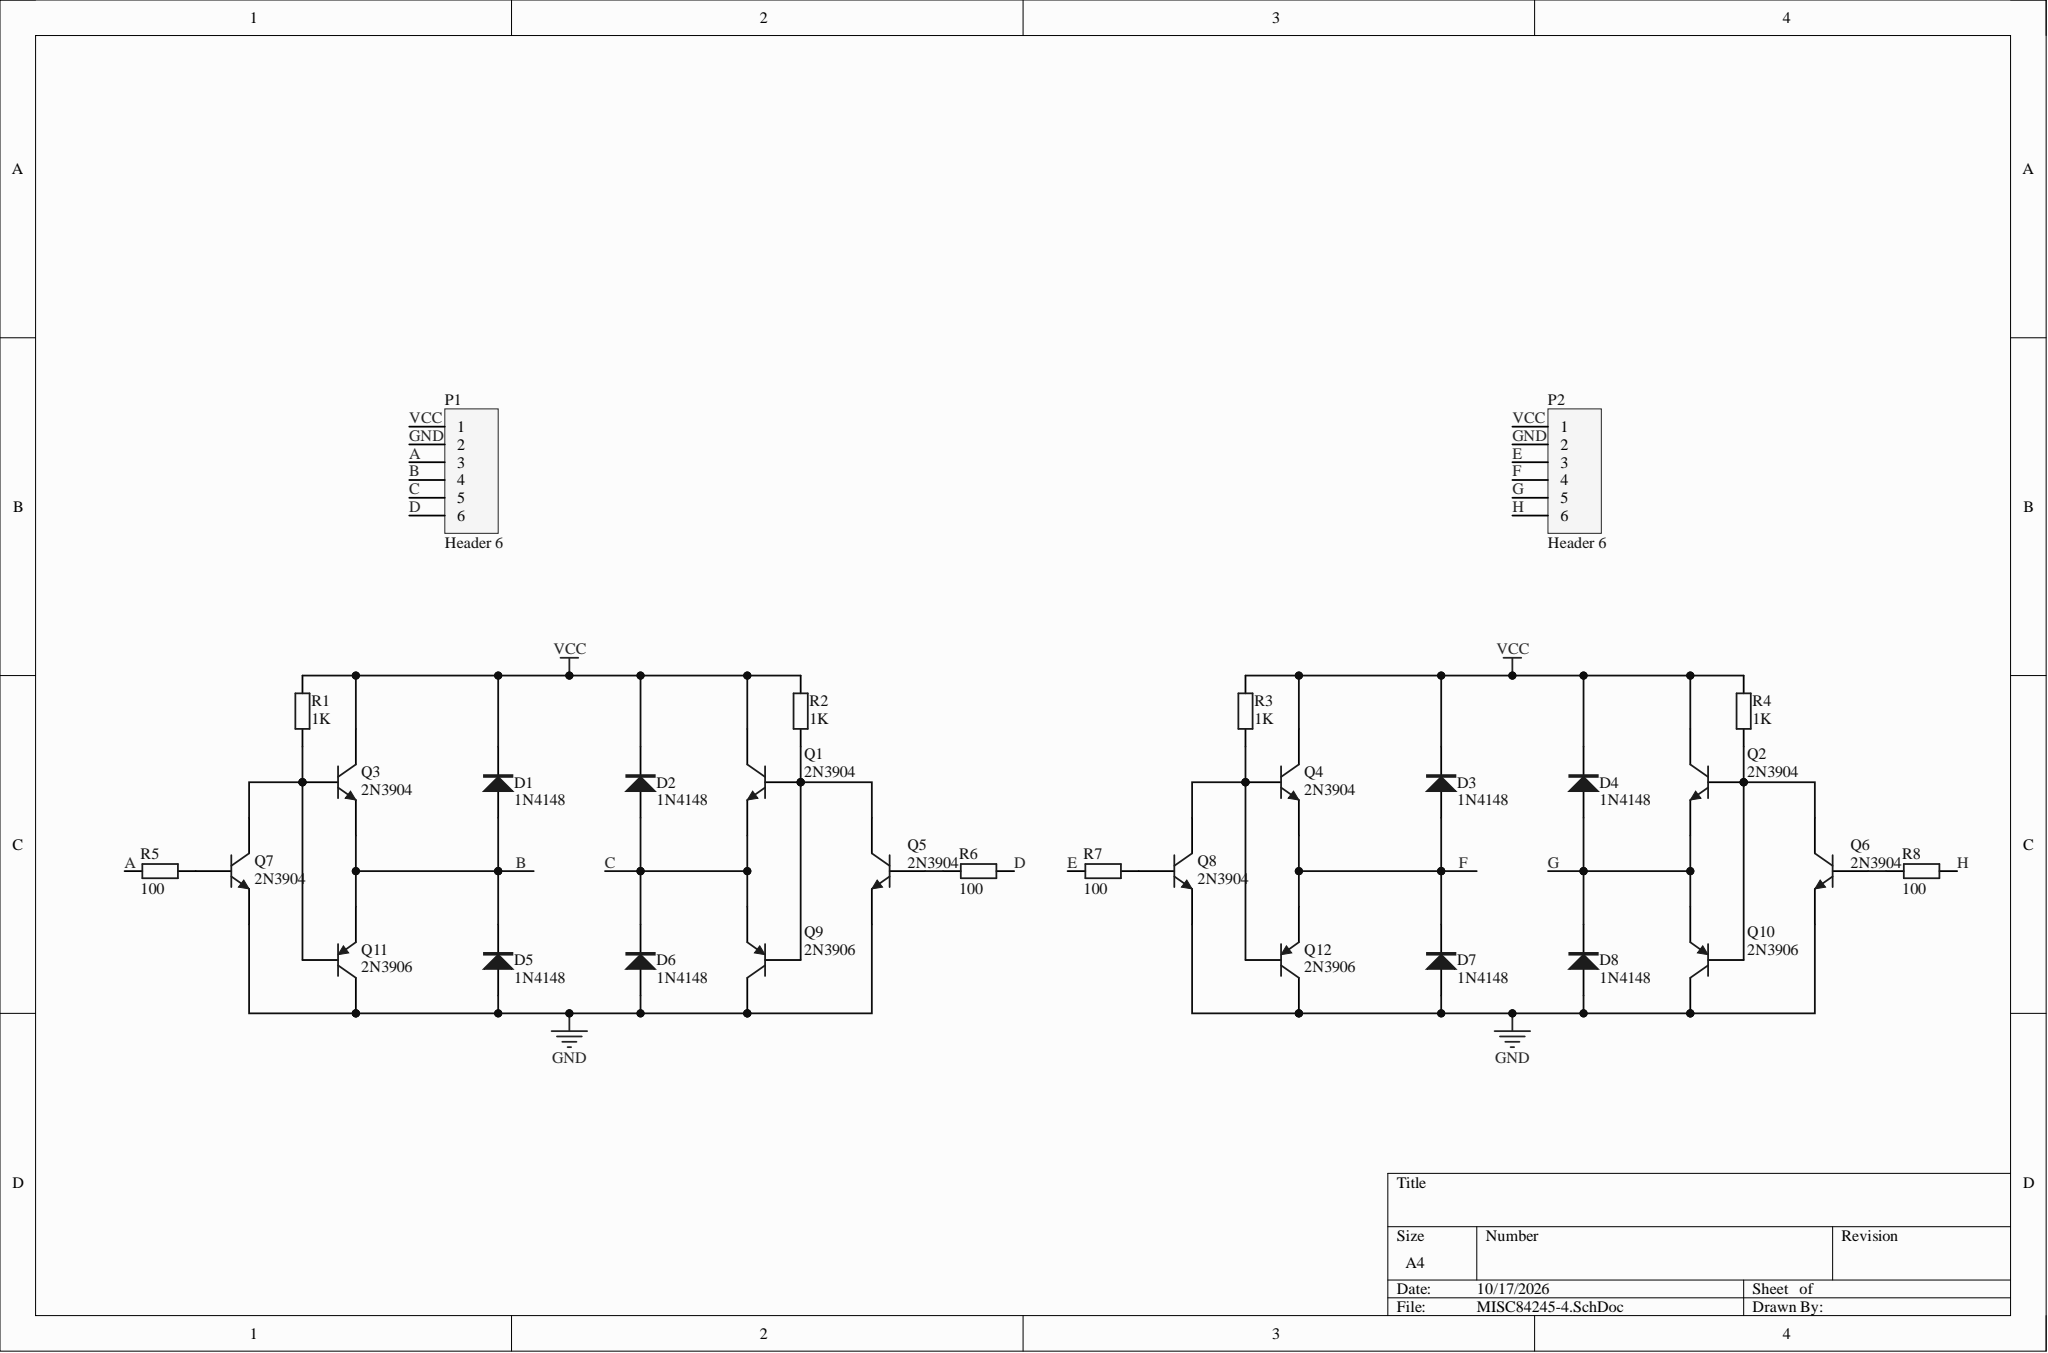Circuit board | Altium Designer | 30 parts | 18 nets
Bill of materials:
Comment,Description,Designator,Footprint,LibRef,Quantity
"1N4148","Switching diode","D1, D2, D3, D4, D5, D6, D7, D8","DO-41","1N4148","8"
"Header 6","Header, 6-Pin","P1, P2","HDR1X6","Header 6","2"
"2N3904","NPN General Purpose Amplifier","Q1, Q2, Q3, Q4, Q5, Q6, Q7, Q8","TO-92A","2N3904","8"
"2N3906","PNP General Purpose Amplifier","Q9, Q10, Q11, Q12","TO-92A","2N3906","4"
"1K","Color-band resistor","R1, R2, R3, R4","RS 1/4W","R-S","4"
"100","Color-band resistor","R5, R6, R7, R8","RS 1/4W","R-S","4"
Netlist (Protel format):
[
D1
DO-41
1N4148



]
[
D2
DO-41
1N4148



]
[
D3
DO-41
1N4148



]
[
D4
DO-41
1N4148



]
[
D5
DO-41
1N4148



]
[
D6
DO-41
1N4148



]
[
D7
DO-41
1N4148



]
[
D8
DO-41
1N4148



]
[
P1
HDR1X6
Header 6



]
[
P2
HDR1X6
Header 6



]
[
Q1
TO-92A
2N3904



]
[
Q2
TO-92A
2N3904



]
[
Q3
TO-92A
2N3904



]
[
Q4
TO-92A
2N3904



]
[
Q5
TO-92A
2N3904



]
[
Q6
TO-92A
2N3904



]
[
Q7
TO-92A
2N3904



]
[
Q8
TO-92A
2N3904



]
[
Q9
TO-92A
2N3906



]
[
Q10
TO-92A
2N3906



]
[
Q11
TO-92A
2N3906



]
[
Q12
TO-92A
2N3906



]
[
R1
RS 1/4W
1K



]
[
R2
RS 1/4W
1K



]
[
R3
RS 1/4W
1K



]
[
R4
RS 1/4W
1K



]
[
R5
RS 1/4W
100



]
[
R6
RS 1/4W
100



]
[
R7
RS 1/4W
100



]
[
R8
RS 1/4W
100



]
(
VCC
D1-2
D2-2
D3-2
D4-2
P1-1
P2-1
Q1-3
Q2-3
Q3-3
Q4-3
R1-2
R2-2
R3-2
R4-2
)
(
NetQ8_2
Q8-2
R7-1
)
(
NetQ7_2
Q7-2
R5-1
)
(
NetQ6_2
Q6-2
R8-2
)
(
NetQ5_2
Q5-2
R6-2
)
(
NetQ4_2
Q4-2
Q8-3
Q12-2
R3-1
)
(
NetQ3_2
Q3-2
Q7-3
Q11-2
R1-1
)
(
NetQ2_2
Q2-2
Q6-3
Q10-2
R4-1
)
(
NetQ1_2
Q1-2
Q5-3
Q9-2
R2-1
)
(
H
P2-6
R8-1
)
(
GND
D5-1
D6-1
D7-1
D8-1
P1-2
P2-2
Q5-1
Q6-1
Q7-1
Q8-1
Q9-3
Q10-3
Q11-3
Q12-3
)
(
G
D4-1
D8-2
P2-5
Q2-1
Q10-1
)
(
F
D3-1
D7-2
P2-4
Q4-1
Q12-1
)
(
E
P2-3
R7-2
)
(
D
P1-6
R6-1
)
(
C
D2-1
D6-2
P1-5
Q1-1
Q9-1
)
(
B
D1-1
D5-2
P1-4
Q3-1
Q11-1
)
(
A
P1-3
R5-2
)